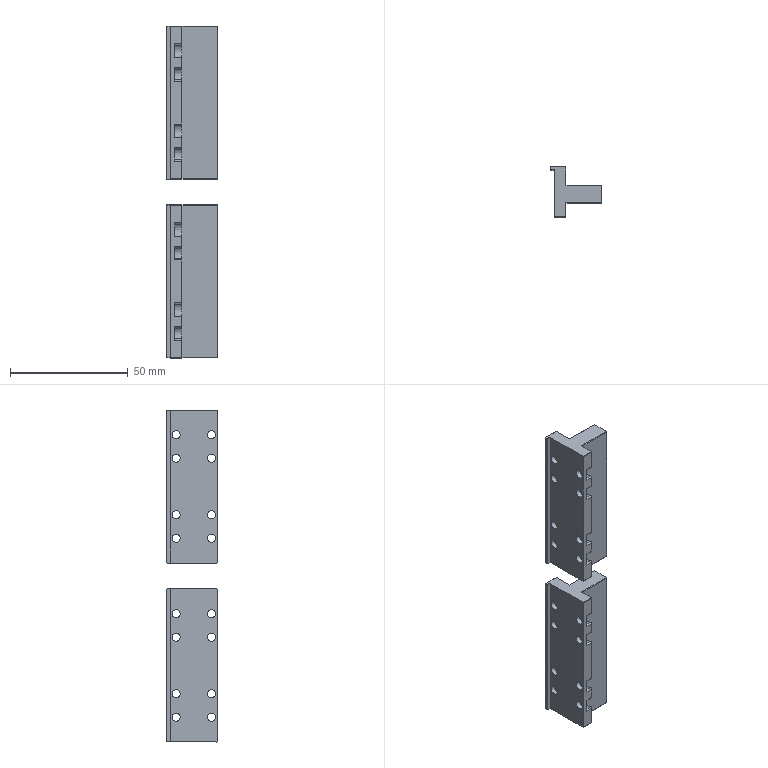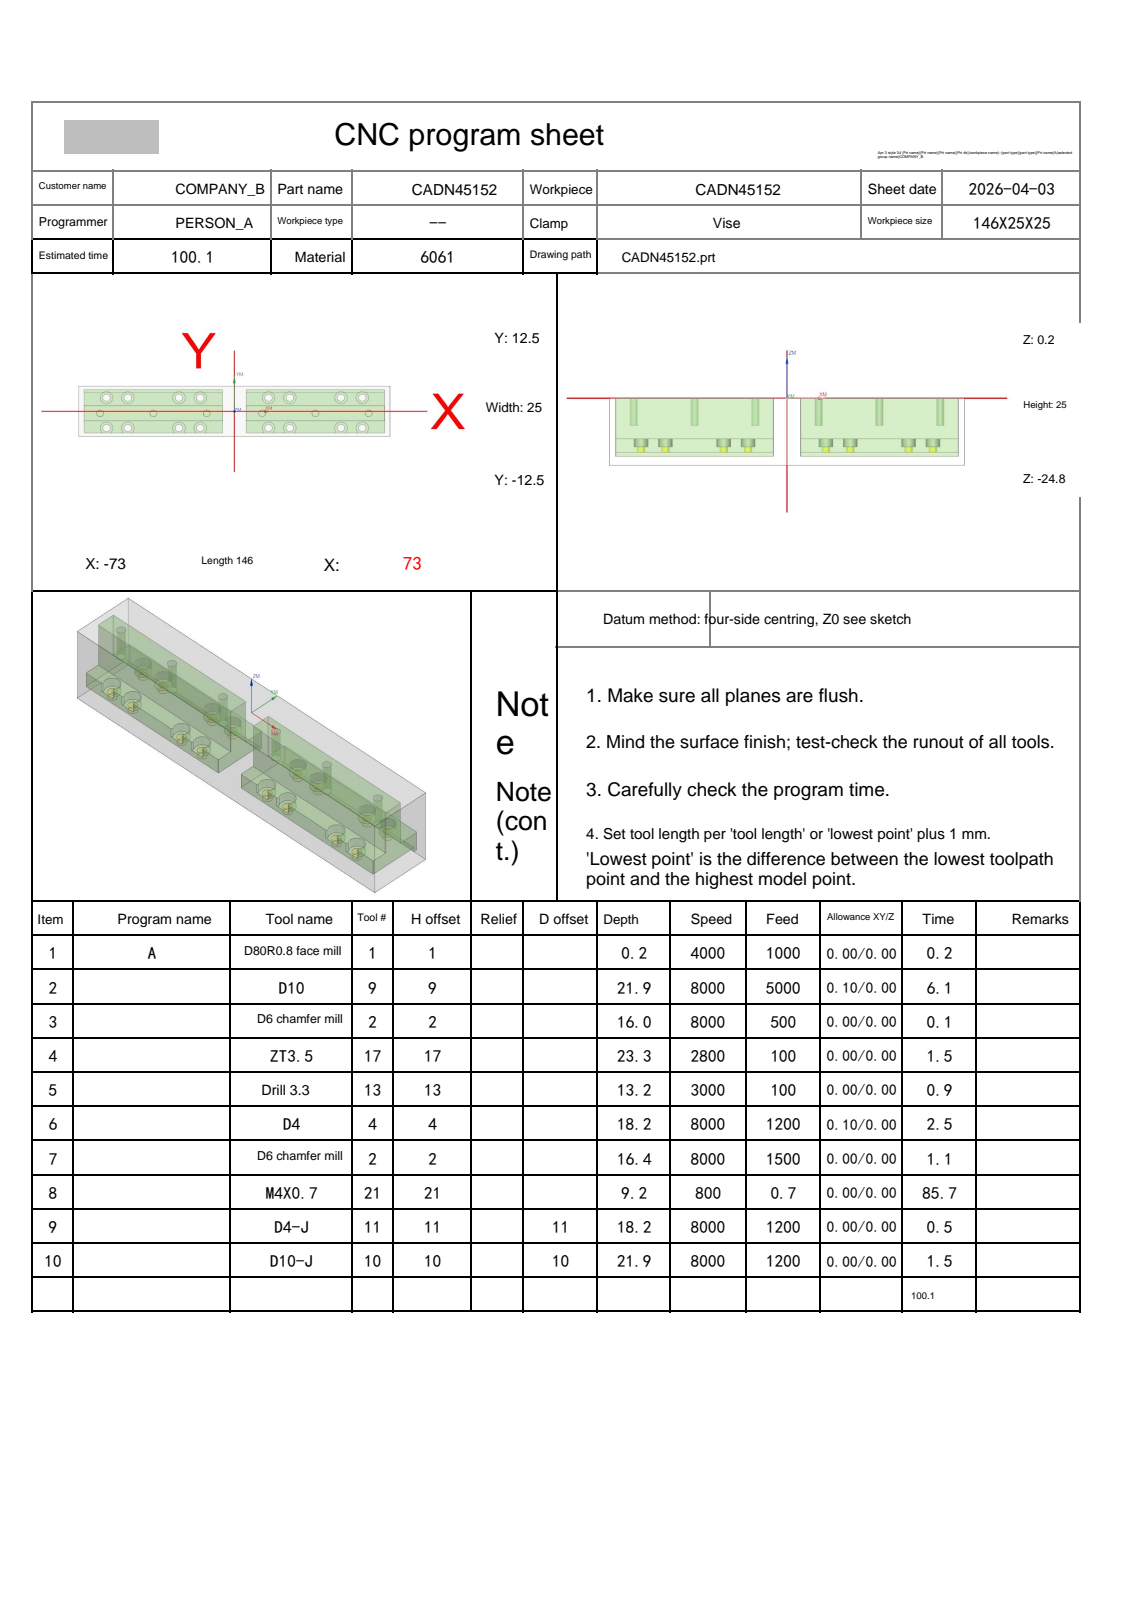NC program | NX | posted by the shop | part box 21.5 x 21.5 x 141 mm
Lines 6087 to 7245 of 7245:
N7 T02 M06
(D6 chamfer mill  D=6. R=0. H=02 ce=0.00 di=0.00)
G00 G90 G54 X-38.386 Y3.977 M03 S6500
G43 H02 Z20.
M08
Z.172
G01 Z-1.199 F1500.
G03 X-38.1 Y3.777 I1.286 J1.532
G01 X-38.054 Y3.747
X-38. Y3.75
X-5.7
X-5.441 Y3.716
X-5.2 Y3.616
X-4.993 Y3.457
X-4.793 Y3.257
X-4.634 Y3.05
X-4.534 Y2.809
X-4.5 Y2.55
Y-4.55
X-4.534 Y-4.809
X-4.634 Y-5.05
X-4.793 Y-5.257
X-4.993 Y-5.457
X-5.2 Y-5.616
X-5.441 Y-5.716
X-5.7 Y-5.75
X-70.3
X-70.559 Y-5.716
X-70.8 Y-5.616
X-71.007 Y-5.457
X-71.207 Y-5.257
X-71.366 Y-5.05
X-71.466 Y-4.809
X-71.5 Y-4.55
Y2.55
X-71.466 Y2.809
X-71.366 Y3.05
X-71.207 Y3.257
X-71.007 Y3.457
X-70.8 Y3.616
X-70.559 Y3.716
X-70.3 Y3.75
X-38.
X-37.946 Y3.747
X-37.9 Y3.777
G03 X-37.614 Y3.977 I-1. J1.732
G01 Z.172
G00 Z10.
X-12.506 Y-1.419
Z.406
G01 Z-1.199
G03 X-12.359 Y-1.103 I-1.732 J1.
G01 X-12.338 Y-1.053
X-12.35 Y-1.
G03 X-13. Y-.35 I-.65 J0.0
X-13.65 Y-1. I0.0 J-.65
X-13. Y-1.65 I.65 J0.0
X-12.35 Y-1. I0.0 J.65
G01 X-12.338 Y-.947
X-12.359 Y-.897
G03 X-12.506 Y-.581 I-1.879 J-.684
G01 Z.402
G00 Z10.
X-37.506 Y-1.419
Z.406
G01 Z-1.199
G03 X-37.359 Y-1.103 I-1.732 J1.
G01 X-37.338 Y-1.053
X-37.35 Y-1.
G03 X-38. Y-.35 I-.65 J0.0
X-38.65 Y-1. I0.0 J-.65
X-38. Y-1.65 I.65 J0.0
X-37.35 Y-1. I0.0 J.65
G01 X-37.338 Y-.947
X-37.359 Y-.897
G03 X-37.506 Y-.581 I-1.879 J-.684
G01 Z.402
G00 Z10.
X-62.506 Y-1.419
Z.406
G01 Z-1.199
G03 X-62.359 Y-1.103 I-1.732 J1.
G01 X-62.338 Y-1.053
X-62.35 Y-1.
G03 X-63. Y-.35 I-.65 J0.0
X-63.65 Y-1. I0.0 J-.65
X-63. Y-1.65 I.65 J0.0
X-62.35 Y-1. I0.0 J.65
G01 X-62.338 Y-.947
X-62.359 Y-.897
G03 X-62.506 Y-.581 I-1.879 J-.684
G01 Z.402
G00 Z10.
X38.386 Y-5.977
Z.172
G01 Z-1.199
G03 X38.1 Y-5.777 I-1.286 J-1.532
G01 X38.054 Y-5.747
X38. Y-5.75
X5.7
X5.441 Y-5.716
X5.2 Y-5.616
X4.993 Y-5.457
X4.793 Y-5.257
X4.634 Y-5.05
X4.534 Y-4.809
X4.5 Y-4.55
Y2.55
X4.534 Y2.809
X4.634 Y3.05
X4.793 Y3.257
X4.993 Y3.457
X5.2 Y3.616
X5.441 Y3.716
X5.7 Y3.75
X70.3
X70.559 Y3.716
X70.8 Y3.616
X71.007 Y3.457
X71.207 Y3.257
X71.366 Y3.05
X71.466 Y2.809
X71.5 Y2.55
Y-4.55
X71.466 Y-4.809
X71.366 Y-5.05
X71.207 Y-5.257
X71.007 Y-5.457
X70.8 Y-5.616
X70.559 Y-5.716
X70.3 Y-5.75
X38.
X37.946 Y-5.747
X37.9 Y-5.777
G03 X37.614 Y-5.977 I1. J-1.732
G01 Z.172
G00 Z10.
X63.494 Y-1.419
Z.406
G01 Z-1.199
G03 X63.641 Y-1.103 I-1.732 J1.
G01 X63.662 Y-1.053
X63.65 Y-1.
G03 X63. Y-.35 I-.65 J0.0
X62.35 Y-1. I0.0 J-.65
X63. Y-1.65 I.65 J0.0
X63.65 Y-1. I0.0 J.65
G01 X63.662 Y-.947
X63.641 Y-.897
G03 X63.494 Y-.581 I-1.879 J-.684
G01 Z.402
G00 Z10.
X38.494 Y-1.419
Z.406
G01 Z-1.199
G03 X38.641 Y-1.103 I-1.732 J1.
G01 X38.662 Y-1.053
X38.65 Y-1.
G03 X38. Y-.35 I-.65 J0.0
X37.35 Y-1. I0.0 J-.65
X38. Y-1.65 I.65 J0.0
X38.65 Y-1. I0.0 J.65
G01 X38.662 Y-.947
X38.641 Y-.897
G03 X38.494 Y-.581 I-1.879 J-.684
G01 Z.402
G00 Z10.
X13.494 Y-1.419
Z.406
G01 Z-1.199
G03 X13.641 Y-1.103 I-1.732 J1.
G01 X13.662 Y-1.053
X13.65 Y-1.
G03 X13. Y-.35 I-.65 J0.0
X12.35 Y-1. I0.0 J-.65
X13. Y-1.65 I.65 J0.0
X13.65 Y-1. I0.0 J.65
G01 X13.662 Y-.947
X13.641 Y-.897
G03 X13.494 Y-.581 I-1.879 J-.684
G01 Z.402
G00 Z10.
X71.591 Y-7.677
Z-1.8
G01 Z-16.199
X71.54 Y-7.727
X71.511 Y-7.791
X71.493 Y-7.808
X71.5 Y-7.831
Y-10.55
X71.466 Y-10.809
X71.366 Y-11.05
X71.207 Y-11.257
X71.007 Y-11.457
X70.8 Y-11.616
X70.559 Y-11.716
X70.3 Y-11.75
X62.872
G02 X61.372 Y-10.25 I0.0 J1.5
X61.641 Y-9.393 I1.5 J0.0
G01 X61.834 Y-9.047
X61.955 Y-8.671
X62. Y-8.278
X61.979 Y-8.032
X61.972 Y-8.012
X61.927 Y-7.959
Z-1.81
G00 Z-1.199
X58.073
Z-1.81
G01 Z-16.199
X58.028 Y-8.012
X58.021 Y-8.032
X58. Y-8.278
X58.045 Y-8.671
X58.166 Y-9.047
X58.359 Y-9.393
G02 X58.628 Y-10.25 I-1.231 J-.857
X57.128 Y-11.75 I-1.5 J0.0
G01 X52.872
G02 X51.372 Y-10.25 I0.0 J1.5
X51.641 Y-9.393 I1.5 J0.0
G01 X51.834 Y-9.047
X51.955 Y-8.671
X52. Y-8.278
X51.979 Y-8.032
X51.972 Y-8.012
X51.927 Y-7.959
Z-1.81
G00 Z-1.199
X48.073
Z-1.81
G01 Z-16.199
X48.028 Y-8.012
X48.021 Y-8.032
X48. Y-8.278
X48.045 Y-8.671
X48.166 Y-9.047
X48.359 Y-9.393
G02 X48.628 Y-10.25 I-1.231 J-.857
X47.128 Y-11.75 I-1.5 J0.0
G01 X28.872
G02 X27.372 Y-10.25 I0.0 J1.5
X27.641 Y-9.393 I1.5 J0.0
G01 X27.834 Y-9.047
X27.955 Y-8.671
X28. Y-8.278
X27.979 Y-8.032
X27.972 Y-8.012
X27.927 Y-7.959
Z-1.81
G00 Z-1.199
X24.073
Z-1.81
G01 Z-16.199
X24.028 Y-8.012
X24.021 Y-8.032
X24. Y-8.278
X24.045 Y-8.671
X24.166 Y-9.047
X24.359 Y-9.393
G02 X24.628 Y-10.25 I-1.231 J-.857
X23.128 Y-11.75 I-1.5 J0.0
G01 X18.872
G02 X17.372 Y-10.25 I0.0 J1.5
X17.641 Y-9.393 I1.5 J0.0
G01 X17.834 Y-9.047
X17.955 Y-8.671
X18. Y-8.278
X17.979 Y-8.032
X17.972 Y-8.012
X17.927 Y-7.959
Z-1.81
G00 Z-1.199
X14.073
Z-1.81
G01 Z-16.199
X14.028 Y-8.012
X14.021 Y-8.032
X14. Y-8.278
X14.045 Y-8.671
X14.166 Y-9.047
X14.359 Y-9.393
G02 X14.628 Y-10.25 I-1.231 J-.857
X13.128 Y-11.75 I-1.5 J0.0
G01 X5.7
X5.441 Y-11.716
X5.2 Y-11.616
X4.993 Y-11.457
X4.793 Y-11.257
X4.634 Y-11.05
X4.534 Y-10.809
X4.5 Y-10.55
Y-7.803
X4.492 Y-7.773
X4.432 Y-7.688
Z-1.801
G00 Z10.
Y5.684
Z-1.798
G01 Z-16.199
X4.492 Y5.77
X4.5 Y5.8
Y10.55
X4.534 Y10.809
X4.634 Y11.05
X4.793 Y11.257
X4.993 Y11.457
X5.2 Y11.616
X5.441 Y11.716
X5.7 Y11.75
X70.3
X70.559 Y11.716
X70.8 Y11.616
X71.007 Y11.457
X71.207 Y11.257
X71.366 Y11.05
X71.466 Y10.809
X71.5 Y10.55
Y5.8
X71.508 Y5.77
X71.568 Y5.684
Z-1.798
G00 Z10.
X17.772 Y5.96
Z-1.812
G01 Z-16.199
X17.854 Y6.026
X17.87 Y6.052
X17.964 Y6.371
G03 X18. Y6.75 I-1.964 J.379
X16. Y8.75 I-2. J0.0
X15.346 Y8.64 I0.0 J-2.
X14.001 Y6.755 I.65 J-1.885
X14.139 Y6.026 I1.994 J0.0
G01 X14.159 Y6.003
X14.25 Y5.95
Z-1.802
G00 Z10.
X27.772 Y5.96
Z-1.812
G01 Z-16.199
X27.854 Y6.026
X27.87 Y6.052
X27.964 Y6.371
G03 X28. Y6.75 I-1.964 J.379
X26. Y8.75 I-2. J0.0
X25.346 Y8.64 I0.0 J-2.
X24.001 Y6.755 I.65 J-1.885
X24.139 Y6.026 I1.994 J0.0
G01 X24.159 Y6.003
X24.25 Y5.95
Z-1.802
G00 Z10.
X51.772 Y5.96
Z-1.812
G01 Z-16.199
X51.854 Y6.026
X51.87 Y6.052
X51.964 Y6.371
G03 X52. Y6.75 I-1.964 J.379
X50. Y8.75 I-2. J0.0
X49.346 Y8.64 I0.0 J-2.
X48.001 Y6.755 I.65 J-1.885
X48.139 Y6.026 I1.994 J0.0
G01 X48.159 Y6.003
X48.25 Y5.95
Z-1.802
G00 Z10.
X61.772 Y5.96
Z-1.812
G01 Z-16.199
X61.854 Y6.026
X61.87 Y6.052
X61.964 Y6.371
G03 X62. Y6.75 I-1.964 J.379
X60. Y8.75 I-2. J0.0
X59.346 Y8.64 I0.0 J-2.
X58.001 Y6.755 I.65 J-1.885
X58.139 Y6.026 I1.994 J0.0
G01 X58.159 Y6.003
X58.25 Y5.95
Z-1.802
G00 Z10.
X-4.409 Y-7.677
Z-1.8
G01 Z-16.199
X-4.46 Y-7.727
X-4.489 Y-7.791
X-4.507 Y-7.808
X-4.5 Y-7.831
Y-10.55
X-4.534 Y-10.809
X-4.634 Y-11.05
X-4.793 Y-11.257
X-4.993 Y-11.457
X-5.2 Y-11.616
X-5.441 Y-11.716
X-5.7 Y-11.75
X-13.128
G02 X-14.628 Y-10.25 I0.0 J1.5
X-14.359 Y-9.393 I1.5 J0.0
G01 X-14.166 Y-9.047
X-14.045 Y-8.671
X-14. Y-8.278
X-14.021 Y-8.032
X-14.028 Y-8.012
X-14.073 Y-7.959
Z-1.81
G00 Z-1.199
X-17.927
Z-1.81
G01 Z-16.199
X-17.972 Y-8.012
X-17.979 Y-8.032
X-18. Y-8.278
X-17.955 Y-8.671
X-17.834 Y-9.047
X-17.641 Y-9.393
G02 X-17.372 Y-10.25 I-1.231 J-.857
X-18.872 Y-11.75 I-1.5 J0.0
G01 X-23.128
G02 X-24.628 Y-10.25 I0.0 J1.5
X-24.359 Y-9.393 I1.5 J0.0
G01 X-24.166 Y-9.047
X-24.045 Y-8.671
X-24. Y-8.278
X-24.021 Y-8.032
X-24.028 Y-8.012
X-24.073 Y-7.959
Z-1.81
G00 Z-1.199
X-27.927
Z-1.81
G01 Z-16.199
X-27.972 Y-8.012
X-27.979 Y-8.032
X-28. Y-8.278
X-27.955 Y-8.671
X-27.834 Y-9.047
X-27.641 Y-9.393
G02 X-27.372 Y-10.25 I-1.231 J-.857
X-28.872 Y-11.75 I-1.5 J0.0
G01 X-47.128
G02 X-48.628 Y-10.25 I0.0 J1.5
X-48.359 Y-9.393 I1.5 J0.0
G01 X-48.166 Y-9.047
X-48.045 Y-8.671
X-48. Y-8.278
X-48.021 Y-8.032
X-48.028 Y-8.012
X-48.073 Y-7.959
Z-1.81
G00 Z-1.199
X-51.927
Z-1.81
G01 Z-16.199
X-51.972 Y-8.012
X-51.979 Y-8.032
X-52. Y-8.278
X-51.955 Y-8.671
X-51.834 Y-9.047
X-51.641 Y-9.393
G02 X-51.372 Y-10.25 I-1.231 J-.857
X-52.872 Y-11.75 I-1.5 J0.0
G01 X-57.128
G02 X-58.628 Y-10.25 I0.0 J1.5
X-58.359 Y-9.393 I1.5 J0.0
G01 X-58.166 Y-9.047
X-58.045 Y-8.671
X-58. Y-8.278
X-58.021 Y-8.032
X-58.028 Y-8.012
X-58.073 Y-7.959
Z-1.81
G00 Z-1.199
X-61.927
Z-1.81
G01 Z-16.199
X-61.972 Y-8.012
X-61.979 Y-8.032
X-62. Y-8.278
X-61.955 Y-8.671
X-61.834 Y-9.047
X-61.641 Y-9.393
G02 X-61.372 Y-10.25 I-1.231 J-.857
X-62.872 Y-11.75 I-1.5 J0.0
G01 X-70.3
X-70.559 Y-11.716
X-70.8 Y-11.616
X-71.007 Y-11.457
X-71.207 Y-11.257
X-71.366 Y-11.05
X-71.466 Y-10.809
X-71.5 Y-10.55
Y-7.803
X-71.508 Y-7.773
X-71.568 Y-7.688
Z-1.801
G00 Z10.
Y5.684
Z-1.798
G01 Z-16.199
X-71.508 Y5.77
X-71.5 Y5.8
Y10.55
X-71.466 Y10.809
X-71.366 Y11.05
X-71.207 Y11.257
X-71.007 Y11.457
X-70.8 Y11.616
X-70.559 Y11.716
X-70.3 Y11.75
X-5.7
X-5.441 Y11.716
X-5.2 Y11.616
X-4.993 Y11.457
X-4.793 Y11.257
X-4.634 Y11.05
X-4.534 Y10.809
X-4.5 Y10.55
Y5.8
X-4.492 Y5.77
X-4.432 Y5.684
Z-1.798
G00 Z10.
X-58.228 Y5.96
Z-1.812
G01 Z-16.199
X-58.146 Y6.026
X-58.13 Y6.052
X-58.036 Y6.371
G03 X-58. Y6.75 I-1.964 J.379
X-60. Y8.75 I-2. J0.0
X-60.654 Y8.64 I0.0 J-2.
X-61.999 Y6.755 I.65 J-1.885
X-61.861 Y6.026 I1.994 J0.0
G01 X-61.841 Y6.003
X-61.75 Y5.95
Z-1.802
G00 Z10.
X-48.228 Y5.96
Z-1.812
G01 Z-16.199
X-48.146 Y6.026
X-48.13 Y6.052
X-48.036 Y6.371
G03 X-48. Y6.75 I-1.964 J.379
X-50. Y8.75 I-2. J0.0
X-50.654 Y8.64 I0.0 J-2.
X-51.999 Y6.755 I.65 J-1.885
X-51.861 Y6.026 I1.994 J0.0
G01 X-51.841 Y6.003
X-51.75 Y5.95
Z-1.802
G00 Z10.
X-24.228 Y5.96
Z-1.812
G01 Z-16.199
X-24.146 Y6.026
X-24.13 Y6.052
X-24.036 Y6.371
G03 X-24. Y6.75 I-1.964 J.379
X-26. Y8.75 I-2. J0.0
X-26.654 Y8.64 I0.0 J-2.
X-27.999 Y6.755 I.65 J-1.885
X-27.861 Y6.026 I1.994 J0.0
G01 X-27.841 Y6.003
X-27.75 Y5.95
Z-1.802
G00 Z10.
X-14.228 Y5.96
Z-1.812
G01 Z-16.199
X-14.146 Y6.026
X-14.13 Y6.052
X-14.036 Y6.371
G03 X-14. Y6.75 I-1.964 J.379
X-16. Y8.75 I-2. J0.0
X-16.654 Y8.64 I0.0 J-2.
X-17.999 Y6.755 I.65 J-1.885
X-17.861 Y6.026 I1.994 J0.0
G01 X-17.841 Y6.003
X-17.75 Y5.95
Z-1.802
G00 Z20.
G00 G90 X63. Y-1. M03 S8000
Z20.
G98 G81 X63. Y-1. Z-2.2 R3. F500.
X38.
X13.
X-13.
X-38.
X-63.
G80
G00 Z20.
G91 G28 Z0.0
M05
M09
G91 G28 Z0.0
M01
N8 T21 M06
(M4X0.7 D=3.3 DR_a=180 H=21)
G00 G90 G54 X63. Y-1. M03 S800
G43 H21 Z20.
M08
G95
G98 G84 X63. Y-1. Z-9. R1. F.7 Q4.
X38.
X13.
X-13.
X-38.
X-63.
G80
G94
G00 Z20.
G91 G28 Z0.0
M05
M09
G91 G28 Z0.0
M01
N9 T11 M06
(D4-J  D=4. R=0. H=11 ce=0.00 di=0.00)
G00 G90 G54 X-60. Y6.75 M03 S8000
G43 H11 Z20.
M08
Z-14.5
G41 D11
G01 X-59.815 Y6.827 F500.
G03 X-59.52 Y7.27 I-.185 J.443
X-60. Y7.75 I-.48 J0.0
X-59.049 Y6.441 Z-18. I0.0 J-1.
X-59. Y6.75 I-.951 J.309
X-60. Y7.75 I-1. J0.0
X-61. Y6.75 I0.0 J-1.
X-60. Y5.75 I1. J0.0
X-59.049 Y6.441 I0.0 J1.
G01 X-59.025 Y6.589
G03 X-59.505 Y7.069 I-.48 J0.0
X-59.87 Y6.902 I0.0 J-.48
G01 G40 X-60. Y6.75
G00 Z20.
X-50.
Z-14.5
G41 D11
G01 X-49.815 Y6.827
G03 X-49.52 Y7.27 I-.185 J.443
X-50. Y7.75 I-.48 J0.0
X-49.049 Y6.441 Z-18. I0.0 J-1.
X-49. Y6.75 I-.951 J.309
X-50. Y7.75 I-1. J0.0
X-51. Y6.75 I0.0 J-1.
X-50. Y5.75 I1. J0.0
X-49.049 Y6.441 I0.0 J1.
G01 X-49.025 Y6.589
G03 X-49.505 Y7.069 I-.48 J0.0
X-49.87 Y6.902 I0.0 J-.48
G01 G40 X-50. Y6.75
G00 Z20.
X-26.
Z-14.5
G41 D11
G01 X-25.815 Y6.827
G03 X-25.52 Y7.27 I-.185 J.443
X-26. Y7.75 I-.48 J0.0
X-25.049 Y6.441 Z-18. I0.0 J-1.
X-25. Y6.75 I-.951 J.309
X-26. Y7.75 I-1. J0.0
X-27. Y6.75 I0.0 J-1.
X-26. Y5.75 I1. J0.0
X-25.049 Y6.441 I0.0 J1.
G01 X-25.025 Y6.589
G03 X-25.505 Y7.069 I-.48 J0.0
X-25.87 Y6.902 I0.0 J-.48
G01 G40 X-26. Y6.75
G00 Z20.
X-16.
Z-14.5
G41 D11
G01 X-15.815 Y6.827
G03 X-15.52 Y7.27 I-.185 J.443
X-16. Y7.75 I-.48 J0.0
X-15.049 Y6.441 Z-18. I0.0 J-1.
X-15. Y6.75 I-.951 J.309
X-16. Y7.75 I-1. J0.0
X-17. Y6.75 I0.0 J-1.
X-16. Y5.75 I1. J0.0
X-15.049 Y6.441 I0.0 J1.
G01 X-15.025 Y6.589
G03 X-15.505 Y7.069 I-.48 J0.0
X-15.87 Y6.902 I0.0 J-.48
G01 G40 X-16. Y6.75
G00 Z20.
X16.
Z-14.5
G41 D11
G01 X16.185 Y6.827
G03 X16.48 Y7.27 I-.185 J.443
X16. Y7.75 I-.48 J0.0
X16.951 Y6.441 Z-18. I0.0 J-1.
X17. Y6.75 I-.951 J.309
X16. Y7.75 I-1. J0.0
X15. Y6.75 I0.0 J-1.
X16. Y5.75 I1. J0.0
X16.951 Y6.441 I0.0 J1.
G01 X16.975 Y6.589
G03 X16.495 Y7.069 I-.48 J0.0
X16.13 Y6.902 I0.0 J-.48
G01 G40 X16. Y6.75
G00 Z20.
X26.
Z-14.5
G41 D11
G01 X26.185 Y6.827
G03 X26.48 Y7.27 I-.185 J.443
X26. Y7.75 I-.48 J0.0
X26.951 Y6.441 Z-18. I0.0 J-1.
X27. Y6.75 I-.951 J.309
X26. Y7.75 I-1. J0.0
X25. Y6.75 I0.0 J-1.
X26. Y5.75 I1. J0.0
X26.951 Y6.441 I0.0 J1.
G01 X26.975 Y6.589
G03 X26.495 Y7.069 I-.48 J0.0
X26.13 Y6.902 I0.0 J-.48
G01 G40 X26. Y6.75
G00 Z20.
X50.
Z-14.5
G41 D11
G01 X50.185 Y6.827
G03 X50.48 Y7.27 I-.185 J.443
X50. Y7.75 I-.48 J0.0
X50.951 Y6.441 Z-18. I0.0 J-1.
X51. Y6.75 I-.951 J.309
X50. Y7.75 I-1. J0.0
X49. Y6.75 I0.0 J-1.
X50. Y5.75 I1. J0.0
X50.951 Y6.441 I0.0 J1.
G01 X50.975 Y6.589
G03 X50.495 Y7.069 I-.48 J0.0
X50.13 Y6.902 I0.0 J-.48
G01 G40 X50. Y6.75
G00 Z20.
X60.
Z-14.5
G41 D11
G01 X60.185 Y6.827
G03 X60.48 Y7.27 I-.185 J.443
X60. Y7.75 I-.48 J0.0
X60.951 Y6.441 Z-18. I0.0 J-1.
X61. Y6.75 I-.951 J.309
X60. Y7.75 I-1. J0.0
X59. Y6.75 I0.0 J-1.
X60. Y5.75 I1. J0.0
X60.951 Y6.441 I0.0 J1.
G01 X60.975 Y6.589
G03 X60.495 Y7.069 I-.48 J0.0
X60.13 Y6.902 I0.0 J-.48
G01 G40 X60. Y6.75
G00 Z20.
G00 G90 X55.172 Y-13.85 M03 S6000
Z20.
Z-17.495
G01 Z-17.995 F1200.
G41 D11
Y-13.25
G03 X54.672 Y-12.75 I-.5 J0.0
G01 X52.872
G02 X50.372 Y-10.25 I0.0 J2.5
X50.821 Y-8.821 I2.5 J0.0
G03 X51. Y-8.25 I-.821 J.571
X50. Y-7.25 I-1. J0.0
X49. Y-8.25 I0.0 J-1.
X49.179 Y-8.821 I1. J0.0
G02 X49.628 Y-10.25 I-2.052 J-1.429
X47.128 Y-12.75 I-2.5 J0.0
G01 X45.328
G03 X44.328 Y-13.75 I0.0 J-1.
G01 G40 Y-13.85
Z-17.495
G00 Z20.
X65.672
Z-17.495
G01 Z-17.995
G41 D11
Y-13.75
G03 X64.672 Y-12.75 I-1. J0.0
G01 X62.872
G02 X60.372 Y-10.25 I0.0 J2.5
X60.821 Y-8.821 I2.5 J0.0
G03 X61. Y-8.25 I-.821 J.571
X60. Y-7.25 I-1. J0.0
X59. Y-8.25 I0.0 J-1.
X59.179 Y-8.821 I1. J0.0
G02 X59.628 Y-10.25 I-2.052 J-1.429
X57.128 Y-12.75 I-2.5 J0.0
G01 X55.328
G03 X54.328 Y-13.75 I0.0 J-1.
G01 G40 Y-13.85
Z-17.495
G00 Z20.
X21.172
Z-17.495
G01 Z-17.995
G41 D11
Y-13.25
G03 X20.672 Y-12.75 I-.5 J0.0
G01 X18.872
G02 X16.372 Y-10.25 I0.0 J2.5
X16.821 Y-8.821 I2.5 J0.0
G03 X17. Y-8.25 I-.821 J.571
X16. Y-7.25 I-1. J0.0
X15. Y-8.25 I0.0 J-1.
X15.179 Y-8.821 I1. J0.0
G02 X15.628 Y-10.25 I-2.052 J-1.429
X13.128 Y-12.75 I-2.5 J0.0
G01 X11.328
G03 X10.328 Y-13.75 I0.0 J-1.
G01 G40 Y-13.85
Z-17.495
G00 Z20.
X31.672
Z-17.495
G01 Z-17.995
G41 D11
Y-13.75
G03 X30.672 Y-12.75 I-1. J0.0
G01 X28.872
G02 X26.372 Y-10.25 I0.0 J2.5
X26.821 Y-8.821 I2.5 J0.0
G03 X27. Y-8.25 I-.821 J.571
X26. Y-7.25 I-1. J0.0
X25. Y-8.25 I0.0 J-1.
X25.179 Y-8.821 I1. J0.0
G02 X25.628 Y-10.25 I-2.052 J-1.429
X23.128 Y-12.75 I-2.5 J0.0
G01 X21.328
G03 X20.328 Y-13.75 I0.0 J-1.
G01 G40 Y-13.85
Z-17.495
G00 Z20.
X-20.828
Z-17.495
G01 Z-17.995
G41 D11
Y-13.25
G03 X-21.328 Y-12.75 I-.5 J0.0
G01 X-23.128
G02 X-25.628 Y-10.25 I0.0 J2.5
X-25.179 Y-8.821 I2.5 J0.0
G03 X-25. Y-8.25 I-.821 J.571
X-26. Y-7.25 I-1. J0.0
X-27. Y-8.25 I0.0 J-1.
X-26.821 Y-8.821 I1. J0.0
G02 X-26.372 Y-10.25 I-2.052 J-1.429
X-28.872 Y-12.75 I-2.5 J0.0
G01 X-30.672
G03 X-31.672 Y-13.75 I0.0 J-1.
G01 G40 Y-13.85
Z-17.495
G00 Z20.
X-10.328
Z-17.495
G01 Z-17.995
G41 D11
Y-13.75
G03 X-11.328 Y-12.75 I-1. J0.0
G01 X-13.128
G02 X-15.628 Y-10.25 I0.0 J2.5
X-15.179 Y-8.821 I2.5 J0.0
G03 X-15. Y-8.25 I-.821 J.571
X-16. Y-7.25 I-1. J0.0
X-17. Y-8.25 I0.0 J-1.
X-16.821 Y-8.821 I1. J0.0
G02 X-16.372 Y-10.25 I-2.052 J-1.429
X-18.872 Y-12.75 I-2.5 J0.0
G01 X-20.672
G03 X-21.672 Y-13.75 I0.0 J-1.
G01 G40 Y-13.85
Z-17.495
G00 Z20.
X-54.828
Z-17.495
G01 Z-17.995
G41 D11
Y-13.25
G03 X-55.328 Y-12.75 I-.5 J0.0
G01 X-57.128
G02 X-59.628 Y-10.25 I0.0 J2.5
X-59.179 Y-8.821 I2.5 J0.0
G03 X-59. Y-8.25 I-.821 J.571
X-60. Y-7.25 I-1. J0.0
X-61. Y-8.25 I0.0 J-1.
X-60.821 Y-8.821 I1. J0.0
G02 X-60.372 Y-10.25 I-2.052 J-1.429
X-62.872 Y-12.75 I-2.5 J0.0
G01 X-64.672
G03 X-65.672 Y-13.75 I0.0 J-1.
G01 G40 Y-13.85
Z-17.495
G00 Z20.
X-44.328
Z-17.495
G01 Z-17.995
G41 D11
Y-13.75
G03 X-45.328 Y-12.75 I-1. J0.0
G01 X-47.128
G02 X-49.628 Y-10.25 I0.0 J2.5
X-49.179 Y-8.821 I2.5 J0.0
G03 X-49. Y-8.25 I-.821 J.571
X-50. Y-7.25 I-1. J0.0
X-51. Y-8.25 I0.0 J-1.
X-50.821 Y-8.821 I1. J0.0
G02 X-50.372 Y-10.25 I-2.052 J-1.429
X-52.872 Y-12.75 I-2.5 J0.0
G01 X-54.672
G03 X-55.672 Y-13.75 I0.0 J-1.
G01 G40 Y-13.85
Z-17.495
G00 Z20.
G91 G28 Z0.0
M05
M09
G91 G28 Z0.0
M01
N10 T10 M06
(D10-J  D=10. R=0. H=10 ce=0.00 di=0.00)
G00 G90 G54 X-76.596 Y4.401 M03 S6000
G43 H10 Z20.
M08
Z-7.
G01 Z-7.5 F1200.
G41 D10
X-76.5 Y4.372
G03 X-76.207 Y4.328 I.293 J.956
X-75.5 Y4.621 I0.0 J1.
G01 X-72.371 Y7.75
X-3.629
X-.5 Y4.621
G03 X-.146 Y4.475 I.354 J.354
X.207 Y4.621 I0.0 J.5
G01 G40 X.278 Y4.692
X-.278
G41 D10
X-.207 Y4.621
G03 X.146 Y4.475 I.354 J.354
X.5 Y4.621 I0.0 J.5
G01 X3.629 Y7.75
X72.371
X75.5 Y4.621
G03 X76.207 Y4.328 I.707 J.707
X76.5 Y4.372 I0.0 J1.
G01 G40 X76.596 Y4.401
Z-7.
G00 Z20.
X0.0 Y5.535
Z-14.5
G01 Z-15.
G41 D10
X-.136 Y4.692
G03 X.217 Y4.545 I.354 J.354
X.571 Y4.692 I0.0 J.5
G01 X3.629 Y7.75
X72.371
X75.429 Y4.692
G03 X76.136 Y4.399 I.707 J.707
X76.5 Y4.467 I0.0 J1.
G01 G40 X76.593 Y4.504
Z-14.5
G00 Z20.
X-76.593
Z-14.5
G01 Z-15.
G41 D10
X-76.5 Y4.467
G03 X-76.136 Y4.399 I.364 J.932
X-75.429 Y4.692 I0.0 J1.
G01 X-72.371 Y7.75
X-3.629
X-.571 Y4.692
G03 X-.217 Y4.545 I.354 J.354
X.136 Y4.692 I0.0 J.5
G01 G40 X0.0 Y5.535
Z-14.5
G00 Z20.
G00 G90 X76.596 Y-6.401 M03 S6000
Z20.
Z-7.
G01 Z-7.5 F1200.
G41 D10
X76.5 Y-6.372
G03 X76.207 Y-6.328 I-.293 J-.956
X75.5 Y-6.621 I0.0 J-1.
G01 X72.371 Y-9.75
X3.629
X.5 Y-6.621
G03 X.146 Y-6.475 I-.354 J-.354
X-.207 Y-6.621 I0.0 J-.5
G01 G40 X-.278 Y-6.692
X.278
G41 D10
X.207 Y-6.621
G03 X-.146 Y-6.475 I-.354 J-.354
X-.5 Y-6.621 I0.0 J-.5
G01 X-3.629 Y-9.75
X-72.371
X-75.5 Y-6.621
G03 X-76.207 Y-6.328 I-.707 J-.707
X-76.5 Y-6.372 I0.0 J-1.
G01 G40 X-76.596 Y-6.401
Z-7.
G00 Z20.
X0.0 Y-7.535
Z-14.5
G01 Z-15.
G41 D10
X.136 Y-6.692
G03 X-.217 Y-6.545 I-.354 J-.354
X-.571 Y-6.692 I0.0 J-.5
G01 X-3.629 Y-9.75
X-72.371
X-75.429 Y-6.692
G03 X-76.136 Y-6.399 I-.707 J-.707
X-76.5 Y-6.467 I0.0 J-1.
G01 G40 X-76.593 Y-6.504
Z-14.5
G00 Z20.
X76.593
Z-14.5
G01 Z-15.
G41 D10
X76.5 Y-6.467
G03 X76.136 Y-6.399 I-.364 J-.932
X75.429 Y-6.692 I0.0 J-1.
G01 X72.371 Y-9.75
X3.629
X.571 Y-6.692
G03 X.217 Y-6.545 I-.354 J-.354
X-.136 Y-6.692 I0.0 J-.5
G01 G40 X0.0 Y-7.535
Z-14.5
G00 Z20.
G00 G90 X-71.3 Y16.95 M03 S8000
Z20.
Z-10.35
G01 Z-10.85 F1000.
G41 D10
Y16.75
G03 X-70.3 Y15.75 I1. J0.0
G01 X-5.7
G02 X-2.164 Y14.286 I0.0 J-5.
G01 X-1.964 Y14.086
G02 X-.5 Y10.55 I-3.536 J-3.536
G01 Y-10.55
G02 X-1.964 Y-14.086 I-5. J0.0
G01 X-2.164 Y-14.286
G02 X-5.7 Y-15.75 I-3.536 J3.536
G01 X-70.3
G02 X-73.836 Y-14.286 I0.0 J5.
G01 X-74.036 Y-14.086
G02 X-75.5 Y-10.55 I3.536 J3.536
G01 Y10.55
G02 X-74.036 Y14.086 I5. J0.0
G01 X-73.836 Y14.286
G02 X-70.3 Y15.75 I3.536 J-3.536
G01 X-69.8
G03 X-68.8 Y16.75 I0.0 J1.
G01 G40 Y16.95
Z-10.35
G00 Z20.
X37.
Z-10.35
G01 Z-10.85
G41 D10
Y16.75
G03 X38. Y15.75 I1. J0.0
G01 X70.3
G02 X73.836 Y14.286 I0.0 J-5.
G01 X74.036 Y14.086
G02 X75.5 Y10.55 I-3.536 J-3.536
G01 Y-10.55
G02 X74.036 Y-14.086 I-5. J0.0
G01 X73.836 Y-14.286
G02 X70.3 Y-15.75 I-3.536 J3.536
G01 X5.7
G02 X2.164 Y-14.286 I0.0 J5.
G01 X1.964 Y-14.086
G02 X.5 Y-10.55 I3.536 J3.536
G01 Y10.55
G02 X1.964 Y14.086 I5. J0.0
G01 X2.164 Y14.286
G02 X5.7 Y15.75 I3.536 J-3.536
G01 X38.
X38.5
G03 X39.5 Y16.75 I0.0 J1.
G01 G40 Y16.95
Z-10.35
G00 Z20.
X4.687 Y16.866
Z-21.2
G01 Z-21.7
G41 D10
X4.703 Y16.667
G03 X5.7 Y15.75 I.997 J.083
G01 X70.3
G02 X73.836 Y14.286 I0.0 J-5.
G01 X74.036 Y14.086
G02 X75.5 Y10.55 I-3.536 J-3.536
G01 Y-10.55
G02 X74.036 Y-14.086 I-5. J0.0
G01 X73.836 Y-14.286
G02 X70.3 Y-15.75 I-3.536 J3.536
G01 X5.7
G02 X2.164 Y-14.286 I0.0 J5.
G01 X1.964 Y-14.086
G02 X.5 Y-10.55 I3.536 J3.536
G01 Y10.55
G02 X1.964 Y14.086 I5. J0.0
G01 X2.164 Y14.286
G02 X5.7 Y15.75 I3.536 J-3.536
G01 X6.2
G03 X7.2 Y16.75 I0.0 J1.
G01 G40 Y16.95
X-.379 Y14.044
G41 D10
X-.553 Y13.945
G03 X-1.058 Y13.077 I.495 J-.869
X-.965 Y12.656 I1. J0.0
G02 X-.5 Y10.55 I-4.535 J-2.106
G01 Y-10.55
G02 X-1.964 Y-14.086 I-5. J0.0
G01 X-2.164 Y-14.286
G02 X-5.7 Y-15.75 I-3.536 J3.536
G01 X-70.3
G02 X-73.836 Y-14.286 I0.0 J5.
G01 X-74.036 Y-14.086
G02 X-75.5 Y-10.55 I3.536 J3.536
G01 Y10.55
G02 X-74.036 Y14.086 I5. J0.0
G01 X-73.836 Y14.286
G02 X-70.3 Y15.75 I3.536 J-3.536
G01 X-5.7
G02 X-2.164 Y14.286 I0.0 J-5.
G01 X-1.964 Y14.086
G02 X-.965 Y12.656 I-3.536 J-3.536
X-.777 Y12.192 I-4.535 J-2.106
G03 X.167 Y11.521 I.945 J.328
X.496 Y11.576 I0.0 J1.
G01 G40 X0.0 Y12.948
Z-21.2
G00 Z20.
M05
M09
G91 G28 Z0.0
G91 G28 Y0.0
M30
%